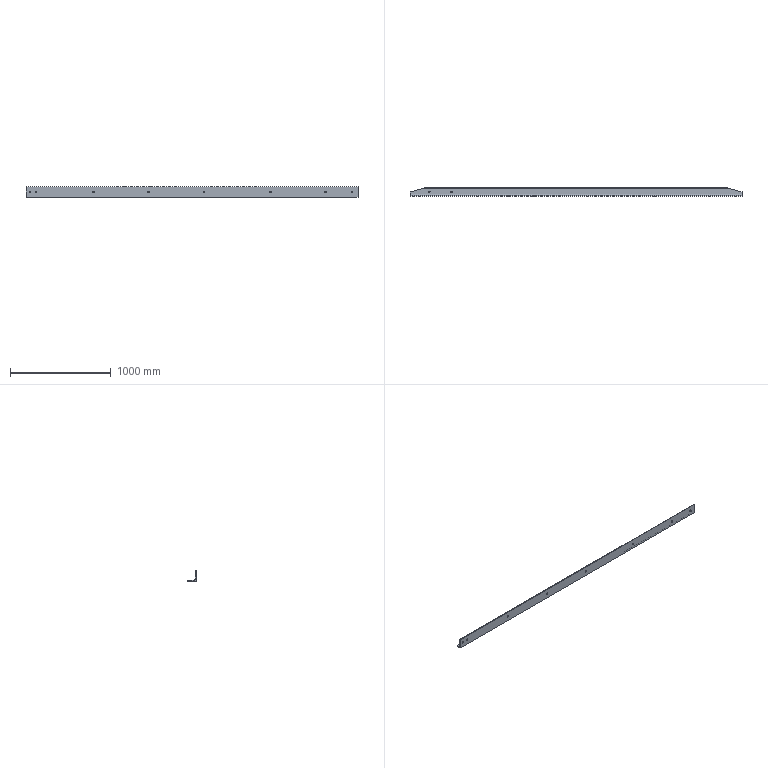Part | SolidWorks | features Chamfer 2, ICE 2, WeldMemberFeat 1, WeldmentFeature 1 | 1 solid | 33 faces | box 3300 x 80 x 100 mm | volume 4536810 mm3 | cylinder 23 | plane 10 | commonest cylinder face diameters 18 x20 5.333 x2 20 x1
STEP:
#1=CARTESIAN_POINT('',(-1469.,40.,8.));
#2=VERTEX_POINT('',#1);
#3=CARTESIAN_POINT('',(-1451.,40.,8.));
#4=VERTEX_POINT('',#3);
#5=CARTESIAN_POINT('',(-1460.,40.,8.));
#6=DIRECTION('',(0.,0.,1.));
#7=DIRECTION('',(0.,1.,0.));
#8=AXIS2_PLACEMENT_3D('',#5,#6,#7);
#9=CIRCLE('',#8,9.);
#10=EDGE_CURVE('',#2,#4,#9,.T.);
#11=ORIENTED_EDGE('',*,*,#10,.T.);
#12=CARTESIAN_POINT('',(-1451.,40.,0.));
#13=VERTEX_POINT('',#12);
#14=CARTESIAN_POINT('',(-1451.,40.,100.001));
#15=DIRECTION('',(0.,0.,-1.));
#16=VECTOR('',#15,1000.);
#17=LINE('',#14,#16);
#18=EDGE_CURVE('',#4,#13,#17,.T.);
#19=ORIENTED_EDGE('',*,*,#18,.T.);
#20=CARTESIAN_POINT('',(-1469.,40.,0.));
#21=VERTEX_POINT('',#20);
#22=CARTESIAN_POINT('',(-1460.,40.,0.));
#23=DIRECTION('',(0.,0.,-1.));
#24=DIRECTION('',(-1.,0.,0.));
#25=AXIS2_PLACEMENT_3D('',#22,#23,#24);
#26=CIRCLE('',#25,9.);
#27=EDGE_CURVE('',#13,#21,#26,.T.);
#28=ORIENTED_EDGE('',*,*,#27,.T.);
#29=CARTESIAN_POINT('',(-1469.,40.,100.001));
#30=DIRECTION('',(0.,0.,-1.));
#31=VECTOR('',#30,1000.);
#32=LINE('',#29,#31);
#33=EDGE_CURVE('',#2,#21,#32,.T.);
#34=ORIENTED_EDGE('',*,*,#33,.F.);
#35=EDGE_LOOP('',(#11,#19,#28,#34));
#36=FACE_OUTER_BOUND('',#35,.T.);
#37=CARTESIAN_POINT('',(-1460.,40.,100.001));
#38=DIRECTION('',(0.,0.,-1.));
#39=DIRECTION('',(-1.,0.,0.));
#40=AXIS2_PLACEMENT_3D('',#37,#38,#39);
#41=CYLINDRICAL_SURFACE('',#40,9.);
#42=ADVANCED_FACE('',(#36),#41,.F.);
#43=CARTESIAN_POINT('',(-1249.,40.,8.));
#44=VERTEX_POINT('',#43);
#45=CARTESIAN_POINT('',(-1231.,40.,8.));
#46=VERTEX_POINT('',#45);
#47=CARTESIAN_POINT('',(-1240.,40.,8.));
#48=DIRECTION('',(0.,0.,1.));
#49=DIRECTION('',(0.,1.,0.));
#50=AXIS2_PLACEMENT_3D('',#47,#48,#49);
#51=CIRCLE('',#50,9.);
#52=EDGE_CURVE('',#44,#46,#51,.T.);
#53=ORIENTED_EDGE('',*,*,#52,.T.);
#54=CARTESIAN_POINT('',(-1231.,40.,0.));
#55=VERTEX_POINT('',#54);
#56=CARTESIAN_POINT('',(-1231.,40.,100.001));
#57=DIRECTION('',(0.,0.,-1.));
#58=VECTOR('',#57,1000.);
#59=LINE('',#56,#58);
#60=EDGE_CURVE('',#46,#55,#59,.T.);
#61=ORIENTED_EDGE('',*,*,#60,.T.);
#62=CARTESIAN_POINT('',(-1249.,40.,0.));
#63=VERTEX_POINT('',#62);
#64=CARTESIAN_POINT('',(-1240.,40.,0.));
#65=DIRECTION('',(0.,0.,-1.));
#66=DIRECTION('',(-1.,0.,0.));
#67=AXIS2_PLACEMENT_3D('',#64,#65,#66);
#68=CIRCLE('',#67,9.);
#69=EDGE_CURVE('',#55,#63,#68,.T.);
#70=ORIENTED_EDGE('',*,*,#69,.T.);
#71=CARTESIAN_POINT('',(-1249.,40.,100.001));
#72=DIRECTION('',(0.,0.,-1.));
#73=VECTOR('',#72,1000.);
#74=LINE('',#71,#73);
#75=EDGE_CURVE('',#44,#63,#74,.T.);
#76=ORIENTED_EDGE('',*,*,#75,.F.);
#77=EDGE_LOOP('',(#53,#61,#70,#76));
#78=FACE_OUTER_BOUND('',#77,.T.);
#79=CARTESIAN_POINT('',(-1240.,40.,100.001));
#80=DIRECTION('',(0.,0.,-1.));
#81=DIRECTION('',(-1.,0.,0.));
#82=AXIS2_PLACEMENT_3D('',#79,#80,#81);
#83=CYLINDRICAL_SURFACE('',#82,9.);
#84=ADVANCED_FACE('',(#78),#83,.F.);
#85=CARTESIAN_POINT('',(-1601.,8.,50.));
#86=VERTEX_POINT('',#85);
#87=CARTESIAN_POINT('',(-1619.,8.,50.));
#88=VERTEX_POINT('',#87);
#89=CARTESIAN_POINT('',(-1610.,8.,50.));
#90=DIRECTION('',(0.,1.,0.));
#91=DIRECTION('',(0.,0.,-1.));
#92=AXIS2_PLACEMENT_3D('',#89,#90,#91);
#93=CIRCLE('',#92,9.);
#94=EDGE_CURVE('',#86,#88,#93,.T.);
#95=ORIENTED_EDGE('',*,*,#94,.T.);
#96=CARTESIAN_POINT('',(-1619.,0.,50.));
#97=VERTEX_POINT('',#96);
#98=CARTESIAN_POINT('',(-1619.,80.001,50.));
#99=DIRECTION('',(0.,-1.,0.));
#100=VECTOR('',#99,1000.);
#101=LINE('',#98,#100);
#102=EDGE_CURVE('',#88,#97,#101,.T.);
#103=ORIENTED_EDGE('',*,*,#102,.T.);
#104=CARTESIAN_POINT('',(-1601.,0.,50.));
#105=VERTEX_POINT('',#104);
#106=CARTESIAN_POINT('',(-1610.,0.,50.));
#107=DIRECTION('',(0.,-1.,0.));
#108=DIRECTION('',(1.,0.,0.));
#109=AXIS2_PLACEMENT_3D('',#106,#107,#108);
#110=CIRCLE('',#109,9.);
#111=EDGE_CURVE('',#97,#105,#110,.T.);
#112=ORIENTED_EDGE('',*,*,#111,.T.);
#113=CARTESIAN_POINT('',(-1601.,80.001,50.));
#114=DIRECTION('',(0.,-1.,0.));
#115=VECTOR('',#114,1000.);
#116=LINE('',#113,#115);
#117=EDGE_CURVE('',#86,#105,#116,.T.);
#118=ORIENTED_EDGE('',*,*,#117,.F.);
#119=EDGE_LOOP('',(#95,#103,#112,#118));
#120=FACE_OUTER_BOUND('',#119,.T.);
#121=CARTESIAN_POINT('',(-1610.,80.001,50.));
#122=DIRECTION('',(0.,-1.,0.));
#123=DIRECTION('',(1.,0.,0.));
#124=AXIS2_PLACEMENT_3D('',#121,#122,#123);
#125=CYLINDRICAL_SURFACE('',#124,9.);
#126=ADVANCED_FACE('',(#120),#125,.F.);
#127=CARTESIAN_POINT('',(-971.,8.,50.));
#128=VERTEX_POINT('',#127);
#129=CARTESIAN_POINT('',(-989.,8.,50.));
#130=VERTEX_POINT('',#129);
#131=CARTESIAN_POINT('',(-980.,8.,50.));
#132=DIRECTION('',(0.,1.,0.));
#133=DIRECTION('',(0.,0.,-1.));
#134=AXIS2_PLACEMENT_3D('',#131,#132,#133);
#135=CIRCLE('',#134,9.);
#136=EDGE_CURVE('',#128,#130,#135,.T.);
#137=ORIENTED_EDGE('',*,*,#136,.T.);
#138=CARTESIAN_POINT('',(-989.,0.,50.));
#139=VERTEX_POINT('',#138);
#140=CARTESIAN_POINT('',(-989.,80.001,50.));
#141=DIRECTION('',(0.,-1.,0.));
#142=VECTOR('',#141,1000.);
#143=LINE('',#140,#142);
#144=EDGE_CURVE('',#130,#139,#143,.T.);
#145=ORIENTED_EDGE('',*,*,#144,.T.);
#146=CARTESIAN_POINT('',(-971.,0.,50.));
#147=VERTEX_POINT('',#146);
#148=CARTESIAN_POINT('',(-980.,0.,50.));
#149=DIRECTION('',(0.,-1.,0.));
#150=DIRECTION('',(1.,0.,0.));
#151=AXIS2_PLACEMENT_3D('',#148,#149,#150);
#152=CIRCLE('',#151,9.);
#153=EDGE_CURVE('',#139,#147,#152,.T.);
#154=ORIENTED_EDGE('',*,*,#153,.T.);
#155=CARTESIAN_POINT('',(-971.,80.001,50.));
#156=DIRECTION('',(0.,-1.,0.));
#157=VECTOR('',#156,1000.);
#158=LINE('',#155,#157);
#159=EDGE_CURVE('',#128,#147,#158,.T.);
#160=ORIENTED_EDGE('',*,*,#159,.F.);
#161=EDGE_LOOP('',(#137,#145,#154,#160));
#162=FACE_OUTER_BOUND('',#161,.T.);
#163=CARTESIAN_POINT('',(-980.,80.001,50.));
#164=DIRECTION('',(0.,-1.,0.));
#165=DIRECTION('',(1.,0.,0.));
#166=AXIS2_PLACEMENT_3D('',#163,#164,#165);
#167=CYLINDRICAL_SURFACE('',#166,9.);
#168=ADVANCED_FACE('',(#162),#167,.F.);
#169=CARTESIAN_POINT('',(-421.,8.,50.));
#170=VERTEX_POINT('',#169);
#171=CARTESIAN_POINT('',(-439.,8.,50.));
#172=VERTEX_POINT('',#171);
#173=CARTESIAN_POINT('',(-430.,8.,50.));
#174=DIRECTION('',(0.,1.,0.));
#175=DIRECTION('',(0.,0.,-1.));
#176=AXIS2_PLACEMENT_3D('',#173,#174,#175);
#177=CIRCLE('',#176,9.);
#178=EDGE_CURVE('',#170,#172,#177,.T.);
#179=ORIENTED_EDGE('',*,*,#178,.T.);
#180=CARTESIAN_POINT('',(-439.,0.,50.));
#181=VERTEX_POINT('',#180);
#182=CARTESIAN_POINT('',(-439.,80.001,50.));
#183=DIRECTION('',(0.,-1.,0.));
#184=VECTOR('',#183,1000.);
#185=LINE('',#182,#184);
#186=EDGE_CURVE('',#172,#181,#185,.T.);
#187=ORIENTED_EDGE('',*,*,#186,.T.);
#188=CARTESIAN_POINT('',(-421.,0.,50.));
#189=VERTEX_POINT('',#188);
#190=CARTESIAN_POINT('',(-430.,0.,50.));
#191=DIRECTION('',(0.,-1.,0.));
#192=DIRECTION('',(1.,0.,0.));
#193=AXIS2_PLACEMENT_3D('',#190,#191,#192);
#194=CIRCLE('',#193,9.);
#195=EDGE_CURVE('',#181,#189,#194,.T.);
#196=ORIENTED_EDGE('',*,*,#195,.T.);
#197=CARTESIAN_POINT('',(-421.,80.001,50.));
#198=DIRECTION('',(0.,-1.,0.));
#199=VECTOR('',#198,1000.);
#200=LINE('',#197,#199);
#201=EDGE_CURVE('',#170,#189,#200,.T.);
#202=ORIENTED_EDGE('',*,*,#201,.F.);
#203=EDGE_LOOP('',(#179,#187,#196,#202));
#204=FACE_OUTER_BOUND('',#203,.T.);
#205=CARTESIAN_POINT('',(-430.,80.001,50.));
#206=DIRECTION('',(0.,-1.,0.));
#207=DIRECTION('',(1.,0.,0.));
#208=AXIS2_PLACEMENT_3D('',#205,#206,#207);
#209=CYLINDRICAL_SURFACE('',#208,9.);
#210=ADVANCED_FACE('',(#204),#209,.F.);
#211=CARTESIAN_POINT('',(129.,8.,50.));
#212=VERTEX_POINT('',#211);
#213=CARTESIAN_POINT('',(111.,8.,50.));
#214=VERTEX_POINT('',#213);
#215=CARTESIAN_POINT('',(120.,8.,50.));
#216=DIRECTION('',(0.,1.,0.));
#217=DIRECTION('',(0.,0.,-1.));
#218=AXIS2_PLACEMENT_3D('',#215,#216,#217);
#219=CIRCLE('',#218,9.);
#220=EDGE_CURVE('',#212,#214,#219,.T.);
#221=ORIENTED_EDGE('',*,*,#220,.T.);
#222=CARTESIAN_POINT('',(111.,0.,50.));
#223=VERTEX_POINT('',#222);
#224=CARTESIAN_POINT('',(111.,80.001,50.));
#225=DIRECTION('',(0.,-1.,0.));
#226=VECTOR('',#225,1000.);
#227=LINE('',#224,#226);
#228=EDGE_CURVE('',#214,#223,#227,.T.);
#229=ORIENTED_EDGE('',*,*,#228,.T.);
#230=CARTESIAN_POINT('',(129.,0.,50.));
#231=VERTEX_POINT('',#230);
#232=CARTESIAN_POINT('',(120.,0.,50.));
#233=DIRECTION('',(0.,-1.,0.));
#234=DIRECTION('',(1.,0.,0.));
#235=AXIS2_PLACEMENT_3D('',#232,#233,#234);
#236=CIRCLE('',#235,9.);
#237=EDGE_CURVE('',#223,#231,#236,.T.);
#238=ORIENTED_EDGE('',*,*,#237,.T.);
#239=CARTESIAN_POINT('',(129.,80.001,50.));
#240=DIRECTION('',(0.,-1.,0.));
#241=VECTOR('',#240,1000.);
#242=LINE('',#239,#241);
#243=EDGE_CURVE('',#212,#231,#242,.T.);
#244=ORIENTED_EDGE('',*,*,#243,.F.);
#245=EDGE_LOOP('',(#221,#229,#238,#244));
#246=FACE_OUTER_BOUND('',#245,.T.);
#247=CARTESIAN_POINT('',(120.,80.001,50.));
#248=DIRECTION('',(0.,-1.,0.));
#249=DIRECTION('',(1.,0.,0.));
#250=AXIS2_PLACEMENT_3D('',#247,#248,#249);
#251=CYLINDRICAL_SURFACE('',#250,9.);
#252=ADVANCED_FACE('',(#246),#251,.F.);
#253=CARTESIAN_POINT('',(-1541.,8.,50.));
#254=VERTEX_POINT('',#253);
#255=CARTESIAN_POINT('',(-1559.,8.,50.));
#256=VERTEX_POINT('',#255);
#257=CARTESIAN_POINT('',(-1550.,8.,50.));
#258=DIRECTION('',(0.,1.,0.));
#259=DIRECTION('',(0.,0.,-1.));
#260=AXIS2_PLACEMENT_3D('',#257,#258,#259);
#261=CIRCLE('',#260,9.);
#262=EDGE_CURVE('',#254,#256,#261,.T.);
#263=ORIENTED_EDGE('',*,*,#262,.T.);
#264=CARTESIAN_POINT('',(-1559.,0.,50.));
#265=VERTEX_POINT('',#264);
#266=CARTESIAN_POINT('',(-1559.,80.001,50.));
#267=DIRECTION('',(0.,-1.,0.));
#268=VECTOR('',#267,1000.);
#269=LINE('',#266,#268);
#270=EDGE_CURVE('',#256,#265,#269,.T.);
#271=ORIENTED_EDGE('',*,*,#270,.T.);
#272=CARTESIAN_POINT('',(-1541.,0.,50.));
#273=VERTEX_POINT('',#272);
#274=CARTESIAN_POINT('',(-1550.,0.,50.));
#275=DIRECTION('',(0.,-1.,0.));
#276=DIRECTION('',(1.,0.,0.));
#277=AXIS2_PLACEMENT_3D('',#274,#275,#276);
#278=CIRCLE('',#277,9.);
#279=EDGE_CURVE('',#265,#273,#278,.T.);
#280=ORIENTED_EDGE('',*,*,#279,.T.);
#281=CARTESIAN_POINT('',(-1541.,80.001,50.));
#282=DIRECTION('',(0.,-1.,0.));
#283=VECTOR('',#282,1000.);
#284=LINE('',#281,#283);
#285=EDGE_CURVE('',#254,#273,#284,.T.);
#286=ORIENTED_EDGE('',*,*,#285,.F.);
#287=EDGE_LOOP('',(#263,#271,#280,#286));
#288=FACE_OUTER_BOUND('',#287,.T.);
#289=CARTESIAN_POINT('',(-1550.,80.001,50.));
#290=DIRECTION('',(0.,-1.,0.));
#291=DIRECTION('',(1.,0.,0.));
#292=AXIS2_PLACEMENT_3D('',#289,#290,#291);
#293=CYLINDRICAL_SURFACE('',#292,9.);
#294=ADVANCED_FACE('',(#288),#293,.F.);
#295=CARTESIAN_POINT('',(1599.,8.,50.));
#296=VERTEX_POINT('',#295);
#297=CARTESIAN_POINT('',(1581.,8.,50.));
#298=VERTEX_POINT('',#297);
#299=CARTESIAN_POINT('',(1590.,8.,50.));
#300=DIRECTION('',(0.,1.,0.));
#301=DIRECTION('',(0.,0.,-1.));
#302=AXIS2_PLACEMENT_3D('',#299,#300,#301);
#303=CIRCLE('',#302,9.);
#304=EDGE_CURVE('',#296,#298,#303,.T.);
#305=ORIENTED_EDGE('',*,*,#304,.T.);
#306=CARTESIAN_POINT('',(1581.,0.,50.));
#307=VERTEX_POINT('',#306);
#308=CARTESIAN_POINT('',(1581.,80.001,50.));
#309=DIRECTION('',(0.,-1.,0.));
#310=VECTOR('',#309,1000.);
#311=LINE('',#308,#310);
#312=EDGE_CURVE('',#298,#307,#311,.T.);
#313=ORIENTED_EDGE('',*,*,#312,.T.);
#314=CARTESIAN_POINT('',(1599.,0.,50.));
#315=VERTEX_POINT('',#314);
#316=CARTESIAN_POINT('',(1590.,0.,50.));
#317=DIRECTION('',(0.,-1.,0.));
#318=DIRECTION('',(1.,0.,0.));
#319=AXIS2_PLACEMENT_3D('',#316,#317,#318);
#320=CIRCLE('',#319,9.);
#321=EDGE_CURVE('',#307,#315,#320,.T.);
#322=ORIENTED_EDGE('',*,*,#321,.T.);
#323=CARTESIAN_POINT('',(1599.,80.001,50.));
#324=DIRECTION('',(0.,-1.,0.));
#325=VECTOR('',#324,1000.);
#326=LINE('',#323,#325);
#327=EDGE_CURVE('',#296,#315,#326,.T.);
#328=ORIENTED_EDGE('',*,*,#327,.F.);
#329=EDGE_LOOP('',(#305,#313,#322,#328));
#330=FACE_OUTER_BOUND('',#329,.T.);
#331=CARTESIAN_POINT('',(1590.,80.001,50.));
#332=DIRECTION('',(0.,-1.,0.));
#333=DIRECTION('',(1.,0.,0.));
#334=AXIS2_PLACEMENT_3D('',#331,#332,#333);
#335=CYLINDRICAL_SURFACE('',#334,9.);
#336=ADVANCED_FACE('',(#330),#335,.F.);
#337=CARTESIAN_POINT('',(1339.,8.,50.));
#338=VERTEX_POINT('',#337);
#339=CARTESIAN_POINT('',(1321.,8.,50.));
#340=VERTEX_POINT('',#339);
#341=CARTESIAN_POINT('',(1330.,8.,50.));
#342=DIRECTION('',(0.,1.,0.));
#343=DIRECTION('',(0.,0.,-1.));
#344=AXIS2_PLACEMENT_3D('',#341,#342,#343);
#345=CIRCLE('',#344,9.);
#346=EDGE_CURVE('',#338,#340,#345,.T.);
#347=ORIENTED_EDGE('',*,*,#346,.T.);
#348=CARTESIAN_POINT('',(1321.,0.,50.));
#349=VERTEX_POINT('',#348);
#350=CARTESIAN_POINT('',(1321.,80.001,50.));
#351=DIRECTION('',(0.,-1.,0.));
#352=VECTOR('',#351,1000.);
#353=LINE('',#350,#352);
#354=EDGE_CURVE('',#340,#349,#353,.T.);
#355=ORIENTED_EDGE('',*,*,#354,.T.);
#356=CARTESIAN_POINT('',(1339.,0.,50.));
#357=VERTEX_POINT('',#356);
#358=CARTESIAN_POINT('',(1330.,0.,50.));
#359=DIRECTION('',(0.,-1.,0.));
#360=DIRECTION('',(1.,0.,0.));
#361=AXIS2_PLACEMENT_3D('',#358,#359,#360);
#362=CIRCLE('',#361,9.);
#363=EDGE_CURVE('',#349,#357,#362,.T.);
#364=ORIENTED_EDGE('',*,*,#363,.T.);
#365=CARTESIAN_POINT('',(1339.,80.001,50.));
#366=DIRECTION('',(0.,-1.,0.));
#367=VECTOR('',#366,1000.);
#368=LINE('',#365,#367);
#369=EDGE_CURVE('',#338,#357,#368,.T.);
#370=ORIENTED_EDGE('',*,*,#369,.F.);
#371=EDGE_LOOP('',(#347,#355,#364,#370));
#372=FACE_OUTER_BOUND('',#371,.T.);
#373=CARTESIAN_POINT('',(1330.,80.001,50.));
#374=DIRECTION('',(0.,-1.,0.));
#375=DIRECTION('',(1.,0.,0.));
#376=AXIS2_PLACEMENT_3D('',#373,#374,#375);
#377=CYLINDRICAL_SURFACE('',#376,9.);
#378=ADVANCED_FACE('',(#372),#377,.F.);
#379=CARTESIAN_POINT('',(789.,8.,50.));
#380=VERTEX_POINT('',#379);
#381=CARTESIAN_POINT('',(771.,8.,50.));
#382=VERTEX_POINT('',#381);
#383=CARTESIAN_POINT('',(780.,8.,50.));
#384=DIRECTION('',(0.,1.,0.));
#385=DIRECTION('',(0.,0.,-1.));
#386=AXIS2_PLACEMENT_3D('',#383,#384,#385);
#387=CIRCLE('',#386,9.);
#388=EDGE_CURVE('',#380,#382,#387,.T.);
#389=ORIENTED_EDGE('',*,*,#388,.T.);
#390=CARTESIAN_POINT('',(771.,0.,50.));
#391=VERTEX_POINT('',#390);
#392=CARTESIAN_POINT('',(771.,80.001,50.));
#393=DIRECTION('',(0.,-1.,0.));
#394=VECTOR('',#393,1000.);
#395=LINE('',#392,#394);
#396=EDGE_CURVE('',#382,#391,#395,.T.);
#397=ORIENTED_EDGE('',*,*,#396,.T.);
#398=CARTESIAN_POINT('',(789.,0.,50.));
#399=VERTEX_POINT('',#398);
#400=CARTESIAN_POINT('',(780.,0.,50.));
#401=DIRECTION('',(0.,-1.,0.));
#402=DIRECTION('',(1.,0.,0.));
#403=AXIS2_PLACEMENT_3D('',#400,#401,#402);
#404=CIRCLE('',#403,9.);
#405=EDGE_CURVE('',#391,#399,#404,.T.);
#406=ORIENTED_EDGE('',*,*,#405,.T.);
#407=CARTESIAN_POINT('',(789.,80.001,50.));
#408=DIRECTION('',(0.,-1.,0.));
#409=VECTOR('',#408,1000.);
#410=LINE('',#407,#409);
#411=EDGE_CURVE('',#380,#399,#410,.T.);
#412=ORIENTED_EDGE('',*,*,#411,.F.);
#413=EDGE_LOOP('',(#389,#397,#406,#412));
#414=FACE_OUTER_BOUND('',#413,.T.);
#415=CARTESIAN_POINT('',(780.,80.001,50.));
#416=DIRECTION('',(0.,-1.,0.));
#417=DIRECTION('',(1.,0.,0.));
#418=AXIS2_PLACEMENT_3D('',#415,#416,#417);
#419=CYLINDRICAL_SURFACE('',#418,9.);
#420=ADVANCED_FACE('',(#414),#419,.F.);
#421=CARTESIAN_POINT('',(-1650.,18.,8.));
#422=VERTEX_POINT('',#421);
#423=CARTESIAN_POINT('',(-1650.,8.,18.));
#424=VERTEX_POINT('',#423);
#425=CARTESIAN_POINT('',(-1650.,18.,18.));
#426=DIRECTION('',(-1.,0.,0.));
#427=DIRECTION('',(0.,0.,-1.));
#428=AXIS2_PLACEMENT_3D('',#425,#426,#427);
#429=CIRCLE('',#428,10.);
#430=EDGE_CURVE('',#422,#424,#429,.T.);
#431=ORIENTED_EDGE('',*,*,#430,.T.);
#432=CARTESIAN_POINT('',(1650.,8.,18.));
#433=VERTEX_POINT('',#432);
#434=CARTESIAN_POINT('',(1650.,8.,18.));
#435=DIRECTION('',(-1.,0.,0.));
#436=VECTOR('',#435,1000.);
#437=LINE('',#434,#436);
#438=EDGE_CURVE('',#433,#424,#437,.T.);
#439=ORIENTED_EDGE('',*,*,#438,.F.);
#440=CARTESIAN_POINT('',(1650.,18.,8.));
#441=VERTEX_POINT('',#440);
#442=CARTESIAN_POINT('',(1650.,18.,18.));
#443=DIRECTION('',(-1.,0.,0.));
#444=DIRECTION('',(0.,0.,-1.));
#445=AXIS2_PLACEMENT_3D('',#442,#443,#444);
#446=CIRCLE('',#445,10.);
#447=EDGE_CURVE('',#441,#433,#446,.T.);
#448=ORIENTED_EDGE('',*,*,#447,.F.);
#449=CARTESIAN_POINT('',(1650.,18.,8.));
#450=DIRECTION('',(-1.,0.,0.));
#451=VECTOR('',#450,1000.);
#452=LINE('',#449,#451);
#453=EDGE_CURVE('',#441,#422,#452,.T.);
#454=ORIENTED_EDGE('',*,*,#453,.T.);
#455=EDGE_LOOP('',(#431,#439,#448,#454));
#456=FACE_OUTER_BOUND('',#455,.T.);
#457=CARTESIAN_POINT('',(1650.,18.,18.));
#458=DIRECTION('',(-1.,0.,0.));
#459=DIRECTION('',(0.,0.,1.));
#460=AXIS2_PLACEMENT_3D('',#457,#458,#459);
#461=CYLINDRICAL_SURFACE('',#460,10.);
#462=ADVANCED_FACE('',(#456),#461,.F.);
#463=ORIENTED_EDGE('',*,*,#94,.F.);
#464=CARTESIAN_POINT('',(-1610.,8.,50.));
#465=DIRECTION('',(0.,1.,0.));
#466=DIRECTION('',(0.,0.,-1.));
#467=AXIS2_PLACEMENT_3D('',#464,#465,#466);
#468=CIRCLE('',#467,9.);
#469=EDGE_CURVE('',#88,#86,#468,.T.);
#470=ORIENTED_EDGE('',*,*,#469,.F.);
#471=EDGE_LOOP('',(#463,#470));
#472=FACE_BOUND('',#471,.T.);
#473=ORIENTED_EDGE('',*,*,#136,.F.);
#474=CARTESIAN_POINT('',(-980.,8.,50.));
#475=DIRECTION('',(0.,1.,0.));
#476=DIRECTION('',(0.,0.,-1.));
#477=AXIS2_PLACEMENT_3D('',#474,#475,#476);
#478=CIRCLE('',#477,9.);
#479=EDGE_CURVE('',#130,#128,#478,.T.);
#480=ORIENTED_EDGE('',*,*,#479,.F.);
#481=EDGE_LOOP('',(#473,#480));
#482=FACE_BOUND('',#481,.T.);
#483=ORIENTED_EDGE('',*,*,#178,.F.);
#484=CARTESIAN_POINT('',(-430.,8.,50.));
#485=DIRECTION('',(0.,1.,0.));
#486=DIRECTION('',(0.,0.,-1.));
#487=AXIS2_PLACEMENT_3D('',#484,#485,#486);
#488=CIRCLE('',#487,9.);
#489=EDGE_CURVE('',#172,#170,#488,.T.);
#490=ORIENTED_EDGE('',*,*,#489,.F.);
#491=EDGE_LOOP('',(#483,#490));
#492=FACE_BOUND('',#491,.T.);
#493=ORIENTED_EDGE('',*,*,#220,.F.);
#494=CARTESIAN_POINT('',(120.,8.,50.));
#495=DIRECTION('',(0.,1.,0.));
#496=DIRECTION('',(0.,0.,-1.));
#497=AXIS2_PLACEMENT_3D('',#494,#495,#496);
#498=CIRCLE('',#497,9.);
#499=EDGE_CURVE('',#214,#212,#498,.T.);
#500=ORIENTED_EDGE('',*,*,#499,.F.);
#501=EDGE_LOOP('',(#493,#500));
#502=FACE_BOUND('',#501,.T.);
#503=ORIENTED_EDGE('',*,*,#262,.F.);
#504=CARTESIAN_POINT('',(-1550.,8.,50.));
#505=DIRECTION('',(0.,1.,0.));
#506=DIRECTION('',(0.,0.,-1.));
#507=AXIS2_PLACEMENT_3D('',#504,#505,#506);
#508=CIRCLE('',#507,9.);
#509=EDGE_CURVE('',#256,#254,#508,.T.);
#510=ORIENTED_EDGE('',*,*,#509,.F.);
#511=EDGE_LOOP('',(#503,#510));
#512=FACE_BOUND('',#511,.T.);
#513=ORIENTED_EDGE('',*,*,#304,.F.);
#514=CARTESIAN_POINT('',(1590.,8.,50.));
#515=DIRECTION('',(0.,1.,0.));
#516=DIRECTION('',(0.,0.,-1.));
#517=AXIS2_PLACEMENT_3D('',#514,#515,#516);
#518=CIRCLE('',#517,9.);
#519=EDGE_CURVE('',#298,#296,#518,.T.);
#520=ORIENTED_EDGE('',*,*,#519,.F.);
#521=EDGE_LOOP('',(#513,#520));
#522=FACE_BOUND('',#521,.T.);
#523=ORIENTED_EDGE('',*,*,#346,.F.);
#524=CARTESIAN_POINT('',(1330.,8.,50.));
#525=DIRECTION('',(0.,1.,0.));
#526=DIRECTION('',(0.,0.,-1.));
#527=AXIS2_PLACEMENT_3D('',#524,#525,#526);
#528=CIRCLE('',#527,9.);
#529=EDGE_CURVE('',#340,#338,#528,.T.);
#530=ORIENTED_EDGE('',*,*,#529,.F.);
#531=EDGE_LOOP('',(#523,#530));
#532=FACE_BOUND('',#531,.T.);
#533=ORIENTED_EDGE('',*,*,#388,.F.);
#534=CARTESIAN_POINT('',(780.,8.,50.));
#535=DIRECTION('',(0.,1.,0.));
#536=DIRECTION('',(0.,0.,-1.));
#537=AXIS2_PLACEMENT_3D('',#534,#535,#536);
#538=CIRCLE('',#537,9.);
#539=EDGE_CURVE('',#382,#380,#538,.T.);
#540=ORIENTED_EDGE('',*,*,#539,.F.);
#541=EDGE_LOOP('',(#533,#540));
#542=FACE_BOUND('',#541,.T.);
#543=CARTESIAN_POINT('',(-1650.,8.,97.333));
#544=VERTEX_POINT('',#543);
#545=CARTESIAN_POINT('',(-1650.,8.,97.333));
#546=DIRECTION('',(0.,0.,1.));
#547=VECTOR('',#546,1000.);
#548=LINE('',#545,#547);
#549=EDGE_CURVE('',#424,#544,#548,.T.);
#550=ORIENTED_EDGE('',*,*,#549,.T.);
#551=CARTESIAN_POINT('',(1650.,8.,97.333));
#552=VERTEX_POINT('',#551);
#553=CARTESIAN_POINT('',(1650.,8.,97.333));
#554=DIRECTION('',(-1.,0.,0.));
#555=VECTOR('',#554,1000.);
#556=LINE('',#553,#555);
#557=EDGE_CURVE('',#552,#544,#556,.T.);
#558=ORIENTED_EDGE('',*,*,#557,.F.);
#559=CARTESIAN_POINT('',(1650.,8.,97.333));
#560=DIRECTION('',(0.,0.,1.));
#561=VECTOR('',#560,1000.);
#562=LINE('',#559,#561);
#563=EDGE_CURVE('',#433,#552,#562,.T.);
#564=ORIENTED_EDGE('',*,*,#563,.F.);
#565=ORIENTED_EDGE('',*,*,#438,.T.);
#566=EDGE_LOOP('',(#550,#558,#564,#565));
#567=FACE_OUTER_BOUND('',#566,.T.);
#568=CARTESIAN_POINT('',(1650.,8.,97.333));
#569=DIRECTION('',(0.,-1.,0.));
#570=DIRECTION('',(0.,0.,-1.));
#571=AXIS2_PLACEMENT_3D('',#568,#569,#570);
#572=PLANE('',#571);
#573=ADVANCED_FACE('',(#472,#482,#492,#502,#512,#522,#532,#542,#567),#572,.F.);
#574=CARTESIAN_POINT('',(-1650.,5.333,100.));
#575=VERTEX_POINT('',#574);
#576=CARTESIAN_POINT('',(-1650.,5.333,97.333));
#577=DIRECTION('',(1.,0.,0.));
#578=DIRECTION('',(0.,0.,1.));
#579=AXIS2_PLACEMENT_3D('',#576,#577,#578);
#580=CIRCLE('',#579,2.667);
#581=EDGE_CURVE('',#544,#575,#580,.T.);
#582=ORIENTED_EDGE('',*,*,#581,.T.);
#583=CARTESIAN_POINT('',(1650.,5.333,100.));
#584=VERTEX_POINT('',#583);
#585=CARTESIAN_POINT('',(1650.,5.333,100.));
#586=DIRECTION('',(-1.,0.,0.));
#587=VECTOR('',#586,1000.);
#588=LINE('',#585,#587);
#589=EDGE_CURVE('',#584,#575,#588,.T.);
#590=ORIENTED_EDGE('',*,*,#589,.F.);
#591=CARTESIAN_POINT('',(1650.,5.333,97.333));
#592=DIRECTION('',(1.,0.,0.));
#593=DIRECTION('',(0.,0.,1.));
#594=AXIS2_PLACEMENT_3D('',#591,#592,#593);
#595=CIRCLE('',#594,2.667);
#596=EDGE_CURVE('',#552,#584,#595,.T.);
#597=ORIENTED_EDGE('',*,*,#596,.F.);
#598=ORIENTED_EDGE('',*,*,#557,.T.);
#599=EDGE_LOOP('',(#582,#590,#597,#598));
#600=FACE_OUTER_BOUND('',#599,.T.);
#601=CARTESIAN_POINT('',(1650.,5.333,97.333));
#602=DIRECTION('',(-1.,0.,0.));
#603=DIRECTION('',(0.,0.,1.));
#604=AXIS2_PLACEMENT_3D('',#601,#602,#603);
#605=CYLINDRICAL_SURFACE('',#604,2.667);
#606=ADVANCED_FACE('',(#600),#605,.T.);
#607=CARTESIAN_POINT('',(-1650.,0.,100.));
#608=VERTEX_POINT('',#607);
#609=CARTESIAN_POINT('',(-1650.,0.,100.));
#610=DIRECTION('',(0.,-1.,0.));
#611=VECTOR('',#610,1000.);
#612=LINE('',#609,#611);
#613=EDGE_CURVE('',#575,#608,#612,.T.);
#614=ORIENTED_EDGE('',*,*,#613,.T.);
#615=CARTESIAN_POINT('',(1650.,0.,100.));
#616=VERTEX_POINT('',#615);
#617=CARTESIAN_POINT('',(1650.,0.,100.));
#618=DIRECTION('',(-1.,0.,0.));
#619=VECTOR('',#618,1000.);
#620=LINE('',#617,#619);
#621=EDGE_CURVE('',#616,#608,#620,.T.);
#622=ORIENTED_EDGE('',*,*,#621,.F.);
#623=CARTESIAN_POINT('',(1650.,0.,100.));
#624=DIRECTION('',(0.,-1.,0.));
#625=VECTOR('',#624,1000.);
#626=LINE('',#623,#625);
#627=EDGE_CURVE('',#584,#616,#626,.T.);
#628=ORIENTED_EDGE('',*,*,#627,.F.);
#629=ORIENTED_EDGE('',*,*,#589,.T.);
#630=EDGE_LOOP('',(#614,#622,#628,#629));
#631=FACE_OUTER_BOUND('',#630,.T.);
#632=CARTESIAN_POINT('',(1650.,0.,100.));
#633=DIRECTION('',(0.,0.,-1.));
#634=DIRECTION('',(0.,1.,0.));
#635=AXIS2_PLACEMENT_3D('',#632,#633,#634);
#636=PLANE('',#635);
#637=ADVANCED_FACE('',(#631),#636,.F.);
#638=CARTESIAN_POINT('',(-1610.,0.,50.));
#639=DIRECTION('',(0.,-1.,0.));
#640=DIRECTION('',(1.,0.,0.));
#641=AXIS2_PLACEMENT_3D('',#638,#639,#640);
#642=CIRCLE('',#641,9.);
#643=EDGE_CURVE('',#105,#97,#642,.T.);
#644=ORIENTED_EDGE('',*,*,#643,.F.);
#645=ORIENTED_EDGE('',*,*,#111,.F.);
#646=EDGE_LOOP('',(#644,#645));
#647=FACE_BOUND('',#646,.T.);
#648=CARTESIAN_POINT('',(-980.,0.,50.));
#649=DIRECTION('',(0.,-1.,0.));
#650=DIRECTION('',(1.,0.,0.));
#651=AXIS2_PLACEMENT_3D('',#648,#649,#650);
#652=CIRCLE('',#651,9.);
#653=EDGE_CURVE('',#147,#139,#652,.T.);
#654=ORIENTED_EDGE('',*,*,#653,.F.);
#655=ORIENTED_EDGE('',*,*,#153,.F.);
#656=EDGE_LOOP('',(#654,#655));
#657=FACE_BOUND('',#656,.T.);
#658=CARTESIAN_POINT('',(-430.,0.,50.));
#659=DIRECTION('',(0.,-1.,0.));
#660=DIRECTION('',(1.,0.,0.));
#661=AXIS2_PLACEMENT_3D('',#658,#659,#660);
#662=CIRCLE('',#661,9.);
#663=EDGE_CURVE('',#189,#181,#662,.T.);
#664=ORIENTED_EDGE('',*,*,#663,.F.);
#665=ORIENTED_EDGE('',*,*,#195,.F.);
#666=EDGE_LOOP('',(#664,#665));
#667=FACE_BOUND('',#666,.T.);
#668=CARTESIAN_POINT('',(120.,0.,50.));
#669=DIRECTION('',(0.,-1.,0.));
#670=DIRECTION('',(1.,0.,0.));
#671=AXIS2_PLACEMENT_3D('',#668,#669,#670);
#672=CIRCLE('',#671,9.);
#673=EDGE_CURVE('',#231,#223,#672,.T.);
#674=ORIENTED_EDGE('',*,*,#673,.F.);
#675=ORIENTED_EDGE('',*,*,#237,.F.);
#676=EDGE_LOOP('',(#674,#675));
#677=FACE_BOUND('',#676,.T.);
#678=CARTESIAN_POINT('',(-1550.,0.,50.));
#679=DIRECTION('',(0.,-1.,0.));
#680=DIRECTION('',(1.,0.,0.));
#681=AXIS2_PLACEMENT_3D('',#678,#679,#680);
#682=CIRCLE('',#681,9.);
#683=EDGE_CURVE('',#273,#265,#682,.T.);
#684=ORIENTED_EDGE('',*,*,#683,.F.);
#685=ORIENTED_EDGE('',*,*,#279,.F.);
#686=EDGE_LOOP('',(#684,#685));
#687=FACE_BOUND('',#686,.T.);
#688=CARTESIAN_POINT('',(1590.,0.,50.));
#689=DIRECTION('',(0.,-1.,0.));
#690=DIRECTION('',(1.,0.,0.));
#691=AXIS2_PLACEMENT_3D('',#688,#689,#690);
#692=CIRCLE('',#691,9.);
#693=EDGE_CURVE('',#315,#307,#692,.T.);
#694=ORIENTED_EDGE('',*,*,#693,.F.);
#695=ORIENTED_EDGE('',*,*,#321,.F.);
#696=EDGE_LOOP('',(#694,#695));
#697=FACE_BOUND('',#696,.T.);
#698=CARTESIAN_POINT('',(1330.,0.,50.));
#699=DIRECTION('',(0.,-1.,0.));
#700=DIRECTION('',(1.,0.,0.));
#701=AXIS2_PLACEMENT_3D('',#698,#699,#700);
#702=CIRCLE('',#701,9.);
#703=EDGE_CURVE('',#357,#349,#702,.T.);
#704=ORIENTED_EDGE('',*,*,#703,.F.);
#705=ORIENTED_EDGE('',*,*,#363,.F.);
#706=EDGE_LOOP('',(#704,#705));
#707=FACE_BOUND('',#706,.T.);
#708=CARTESIAN_POINT('',(780.,0.,50.));
#709=DIRECTION('',(0.,-1.,0.));
#710=DIRECTION('',(1.,0.,0.));
#711=AXIS2_PLACEMENT_3D('',#708,#709,#710);
#712=CIRCLE('',#711,9.);
#713=EDGE_CURVE('',#399,#391,#712,.T.);
#714=ORIENTED_EDGE('',*,*,#713,.F.);
#715=ORIENTED_EDGE('',*,*,#405,.F.);
#716=EDGE_LOOP('',(#714,#715));
#717=FACE_BOUND('',#716,.T.);
#718=CARTESIAN_POINT('',(-1650.,0.,0.));
#719=VERTEX_POINT('',#718);
#720=CARTESIAN_POINT('',(-1650.,0.,100.));
#721=DIRECTION('',(0.,0.,-1.));
#722=VECTOR('',#721,1000.);
#723=LINE('',#720,#722);
#724=EDGE_CURVE('',#608,#719,#723,.T.);
#725=ORIENTED_EDGE('',*,*,#724,.T.);
#726=CARTESIAN_POINT('',(1650.,0.,0.));
#727=VERTEX_POINT('',#726);
#728=CARTESIAN_POINT('',(1650.,0.,0.));
#729=DIRECTION('',(-1.,0.,0.));
#730=VECTOR('',#729,1000.);
#731=LINE('',#728,#730);
#732=EDGE_CURVE('',#727,#719,#731,.T.);
#733=ORIENTED_EDGE('',*,*,#732,.F.);
#734=CARTESIAN_POINT('',(1650.,0.,100.));
#735=DIRECTION('',(0.,0.,-1.));
#736=VECTOR('',#735,1000.);
#737=LINE('',#734,#736);
#738=EDGE_CURVE('',#616,#727,#737,.T.);
#739=ORIENTED_EDGE('',*,*,#738,.F.);
#740=ORIENTED_EDGE('',*,*,#621,.T.);
#741=EDGE_LOOP('',(#725,#733,#739,#740));
#742=FACE_OUTER_BOUND('',#741,.T.);
#743=CARTESIAN_POINT('',(1650.,0.,100.));
#744=DIRECTION('',(0.,1.,0.));
#745=DIRECTION('',(0.,0.,1.));
#746=AXIS2_PLACEMENT_3D('',#743,#744,#745);
#747=PLANE('',#746);
#748=ADVANCED_FACE('',(#647,#657,#667,#677,#687,#697,#707,#717,#742),#747,.F.);
#749=CARTESIAN_POINT('',(-1460.,40.,0.));
#750=DIRECTION('',(0.,0.,-1.));
#751=DIRECTION('',(-1.,0.,0.));
#752=AXIS2_PLACEMENT_3D('',#749,#750,#751);
#753=CIRCLE('',#752,9.);
#754=EDGE_CURVE('',#21,#13,#753,.T.);
#755=ORIENTED_EDGE('',*,*,#754,.F.);
#756=ORIENTED_EDGE('',*,*,#27,.F.);
#757=EDGE_LOOP('',(#755,#756));
#758=FACE_BOUND('',#757,.T.);
#759=CARTESIAN_POINT('',(-1240.,40.,0.));
#760=DIRECTION('',(0.,0.,-1.));
#761=DIRECTION('',(-1.,0.,0.));
#762=AXIS2_PLACEMENT_3D('',#759,#760,#761);
#763=CIRCLE('',#762,9.);
#764=EDGE_CURVE('',#63,#55,#763,.T.);
#765=ORIENTED_EDGE('',*,*,#764,.F.);
#766=ORIENTED_EDGE('',*,*,#69,.F.);
#767=EDGE_LOOP('',(#765,#766));
#768=FACE_BOUND('',#767,.T.);
#769=CARTESIAN_POINT('',(1510.,80.,0.));
#770=VERTEX_POINT('',#769);
#771=CARTESIAN_POINT('',(-1510.,80.,0.));
#772=VERTEX_POINT('',#771);
#773=CARTESIAN_POINT('',(1650.,80.,0.));
#774=DIRECTION('',(-1.,0.,0.));
#775=VECTOR('',#774,1000.);
#776=LINE('',#773,#775);
#777=EDGE_CURVE('',#770,#772,#776,.T.);
#778=ORIENTED_EDGE('',*,*,#777,.F.);
#779=CARTESIAN_POINT('',(1650.,40.,0.));
#780=VERTEX_POINT('',#779);
#781=CARTESIAN_POINT('',(1650.,40.,0.));
#782=DIRECTION('',(0.9615,-0.2747,0.));
#783=VECTOR('',#782,1000.);
#784=LINE('',#781,#783);
#785=EDGE_CURVE('',#770,#780,#784,.T.);
#786=ORIENTED_EDGE('',*,*,#785,.T.);
#787=CARTESIAN_POINT('',(1650.,0.,0.));
#788=DIRECTION('',(0.,1.,0.));
#789=VECTOR('',#788,1000.);
#790=LINE('',#787,#789);
#791=EDGE_CURVE('',#727,#780,#790,.T.);
#792=ORIENTED_EDGE('',*,*,#791,.F.);
#793=ORIENTED_EDGE('',*,*,#732,.T.);
#794=CARTESIAN_POINT('',(-1650.,40.,0.));
#795=VERTEX_POINT('',#794);
#796=CARTESIAN_POINT('',(-1650.,0.,0.));
#797=DIRECTION('',(0.,1.,0.));
#798=VECTOR('',#797,1000.);
#799=LINE('',#796,#798);
#800=EDGE_CURVE('',#719,#795,#799,.T.);
#801=ORIENTED_EDGE('',*,*,#800,.T.);
#802=CARTESIAN_POINT('',(-1510.,80.,0.));
#803=DIRECTION('',(0.9615,0.2747,0.));
#804=VECTOR('',#803,1000.);
#805=LINE('',#802,#804);
#806=EDGE_CURVE('',#795,#772,#805,.T.);
#807=ORIENTED_EDGE('',*,*,#806,.T.);
#808=EDGE_LOOP('',(#778,#786,#792,#793,#801,#807));
#809=FACE_OUTER_BOUND('',#808,.T.);
#810=CARTESIAN_POINT('',(1650.,0.,0.));
#811=DIRECTION('',(0.,0.,1.));
#812=DIRECTION('',(1.,0.,0.));
#813=AXIS2_PLACEMENT_3D('',#810,#811,#812);
#814=PLANE('',#813);
#815=ADVANCED_FACE('',(#758,#768,#809),#814,.F.);
#816=CARTESIAN_POINT('',(1510.,80.,5.333));
#817=VERTEX_POINT('',#816);
#818=CARTESIAN_POINT('',(-1510.,80.,5.333));
#819=VERTEX_POINT('',#818);
#820=CARTESIAN_POINT('',(1650.,80.,5.333));
#821=DIRECTION('',(-1.,0.,0.));
#822=VECTOR('',#821,1000.);
#823=LINE('',#820,#822);
#824=EDGE_CURVE('',#817,#819,#823,.T.);
#825=ORIENTED_EDGE('',*,*,#824,.F.);
#826=CARTESIAN_POINT('',(1510.,80.,0.));
#827=DIRECTION('',(0.,0.,-1.));
#828=VECTOR('',#827,1000.);
#829=LINE('',#826,#828);
#830=EDGE_CURVE('',#817,#770,#829,.T.);
#831=ORIENTED_EDGE('',*,*,#830,.T.);
#832=ORIENTED_EDGE('',*,*,#777,.T.);
#833=CARTESIAN_POINT('',(-1510.,80.,0.));
#834=DIRECTION('',(0.,0.,1.));
#835=VECTOR('',#834,1000.);
#836=LINE('',#833,#835);
#837=EDGE_CURVE('',#772,#819,#836,.T.);
#838=ORIENTED_EDGE('',*,*,#837,.T.);
#839=EDGE_LOOP('',(#825,#831,#832,#838));
#840=FACE_OUTER_BOUND('',#839,.T.);
#841=CARTESIAN_POINT('',(1650.,80.,0.));
#842=DIRECTION('',(0.,-1.,0.));
#843=DIRECTION('',(0.,0.,-1.));
#844=AXIS2_PLACEMENT_3D('',#841,#842,#843);
#845=PLANE('',#844);
#846=ADVANCED_FACE('',(#840),#845,.F.);
#847=CARTESIAN_POINT('',(1519.333,77.333,8.));
#848=VERTEX_POINT('',#847);
#849=CARTESIAN_POINT('',(-1519.333,77.333,8.));
#850=VERTEX_POINT('',#849);
#851=CARTESIAN_POINT('',(1650.,77.333,8.));
#852=DIRECTION('',(-1.,0.,0.));
#853=VECTOR('',#852,1000.);
#854=LINE('',#851,#853);
#855=EDGE_CURVE('',#848,#850,#854,.T.);
#856=ORIENTED_EDGE('',*,*,#855,.F.);
#857=CARTESIAN_POINT('',(1519.333,77.333,8.));
#858=CARTESIAN_POINT('',(1513.866,78.895,8.));
#859=CARTESIAN_POINT('',(1510.,80.,6.895));
#860=CARTESIAN_POINT('',(1510.,80.,5.333));
#861=(BOUNDED_CURVE()B_SPLINE_CURVE(3,(#857,#858,#859,#860),.UNSPECIFIED.,.F.,.F.)B_SPLINE_CURVE_WITH_KNOTS((4,4),(4.712,6.283),.UNSPECIFIED.)CURVE()GEOMETRIC_REPRESENTATION_ITEM()RATIONAL_B_SPLINE_CURVE((1.,0.8047,0.8047,1.))REPRESENTATION_ITEM(''));
#862=EDGE_CURVE('',#848,#817,#861,.T.);
#863=ORIENTED_EDGE('',*,*,#862,.T.);
#864=ORIENTED_EDGE('',*,*,#824,.T.);
#865=CARTESIAN_POINT('',(-1510.,80.,5.333));
#866=CARTESIAN_POINT('',(-1510.,80.,6.895));
#867=CARTESIAN_POINT('',(-1513.866,78.895,8.));
#868=CARTESIAN_POINT('',(-1519.333,77.333,8.));
#869=(BOUNDED_CURVE()B_SPLINE_CURVE(3,(#865,#866,#867,#868),.UNSPECIFIED.,.F.,.F.)B_SPLINE_CURVE_WITH_KNOTS((4,4),(3.142,4.712),.UNSPECIFIED.)CURVE()GEOMETRIC_REPRESENTATION_ITEM()RATIONAL_B_SPLINE_CURVE((1.,0.8047,0.8047,1.))REPRESENTATION_ITEM(''));
#870=EDGE_CURVE('',#819,#850,#869,.T.);
#871=ORIENTED_EDGE('',*,*,#870,.T.);
#872=EDGE_LOOP('',(#856,#863,#864,#871));
#873=FACE_OUTER_BOUND('',#872,.T.);
#874=CARTESIAN_POINT('',(1650.,77.333,5.333));
#875=DIRECTION('',(-1.,0.,0.));
#876=DIRECTION('',(0.,0.,1.));
#877=AXIS2_PLACEMENT_3D('',#874,#875,#876);
#878=CYLINDRICAL_SURFACE('',#877,2.667);
#879=ADVANCED_FACE('',(#873),#878,.T.);
#880=ORIENTED_EDGE('',*,*,#10,.F.);
#881=CARTESIAN_POINT('',(-1460.,40.,8.));
#882=DIRECTION('',(0.,0.,1.));
#883=DIRECTION('',(0.,1.,0.));
#884=AXIS2_PLACEMENT_3D('',#881,#882,#883);
#885=CIRCLE('',#884,9.);
#886=EDGE_CURVE('',#4,#2,#885,.T.);
#887=ORIENTED_EDGE('',*,*,#886,.F.);
#888=EDGE_LOOP('',(#880,#887));
#889=FACE_BOUND('',#888,.T.);
#890=ORIENTED_EDGE('',*,*,#52,.F.);
#891=CARTESIAN_POINT('',(-1240.,40.,8.));
#892=DIRECTION('',(0.,0.,1.));
#893=DIRECTION('',(0.,1.,0.));
#894=AXIS2_PLACEMENT_3D('',#891,#892,#893);
#895=CIRCLE('',#894,9.);
#896=EDGE_CURVE('',#46,#44,#895,.T.);
#897=ORIENTED_EDGE('',*,*,#896,.F.);
#898=EDGE_LOOP('',(#890,#897));
#899=FACE_BOUND('',#898,.T.);
#900=CARTESIAN_POINT('',(1650.,40.,8.));
#901=VERTEX_POINT('',#900);
#902=CARTESIAN_POINT('',(1650.,18.,8.));
#903=DIRECTION('',(0.,-1.,0.));
#904=VECTOR('',#903,1000.);
#905=LINE('',#902,#904);
#906=EDGE_CURVE('',#901,#441,#905,.T.);
#907=ORIENTED_EDGE('',*,*,#906,.F.);
#908=CARTESIAN_POINT('',(1650.,40.,8.));
#909=DIRECTION('',(-0.9615,0.2747,0.));
#910=VECTOR('',#909,1000.);
#911=LINE('',#908,#910);
#912=EDGE_CURVE('',#901,#848,#911,.T.);
#913=ORIENTED_EDGE('',*,*,#912,.T.);
#914=ORIENTED_EDGE('',*,*,#855,.T.);
#915=CARTESIAN_POINT('',(-1650.,40.,8.));
#916=VERTEX_POINT('',#915);
#917=CARTESIAN_POINT('',(-1510.,80.,8.));
#918=DIRECTION('',(-0.9615,-0.2747,0.));
#919=VECTOR('',#918,1000.);
#920=LINE('',#917,#919);
#921=EDGE_CURVE('',#850,#916,#920,.T.);
#922=ORIENTED_EDGE('',*,*,#921,.T.);
#923=CARTESIAN_POINT('',(-1650.,18.,8.));
#924=DIRECTION('',(0.,-1.,0.));
#925=VECTOR('',#924,1000.);
#926=LINE('',#923,#925);
#927=EDGE_CURVE('',#916,#422,#926,.T.);
#928=ORIENTED_EDGE('',*,*,#927,.T.);
#929=ORIENTED_EDGE('',*,*,#453,.F.);
#930=EDGE_LOOP('',(#907,#913,#914,#922,#928,#929));
#931=FACE_OUTER_BOUND('',#930,.T.);
#932=CARTESIAN_POINT('',(1650.,18.,8.));
#933=DIRECTION('',(0.,0.,-1.));
#934=DIRECTION('',(0.,1.,0.));
#935=AXIS2_PLACEMENT_3D('',#932,#933,#934);
#936=PLANE('',#935);
#937=ADVANCED_FACE('',(#889,#899,#931),#936,.F.);
#938=ORIENTED_EDGE('',*,*,#791,.T.);
#939=CARTESIAN_POINT('',(1650.,40.,5.333));
#940=DIRECTION('',(0.,0.,1.));
#941=VECTOR('',#940,1000.);
#942=LINE('',#939,#941);
#943=EDGE_CURVE('',#780,#901,#942,.T.);
#944=ORIENTED_EDGE('',*,*,#943,.T.);
#945=ORIENTED_EDGE('',*,*,#906,.T.);
#946=ORIENTED_EDGE('',*,*,#447,.T.);
#947=ORIENTED_EDGE('',*,*,#563,.T.);
#948=ORIENTED_EDGE('',*,*,#596,.T.);
#949=ORIENTED_EDGE('',*,*,#627,.T.);
#950=ORIENTED_EDGE('',*,*,#738,.T.);
#951=EDGE_LOOP('',(#938,#944,#945,#946,#947,#948,#949,#950));
#952=FACE_OUTER_BOUND('',#951,.T.);
#953=CARTESIAN_POINT('',(1650.,18.,18.));
#954=DIRECTION('',(1.,0.,0.));
#955=DIRECTION('',(0.,0.,-1.));
#956=AXIS2_PLACEMENT_3D('',#953,#954,#955);
#957=PLANE('',#956);
#958=ADVANCED_FACE('',(#952),#957,.T.);
#959=ORIENTED_EDGE('',*,*,#927,.F.);
#960=CARTESIAN_POINT('',(-1650.,40.,18.));
#961=DIRECTION('',(0.,0.,-1.));
#962=VECTOR('',#961,1000.);
#963=LINE('',#960,#962);
#964=EDGE_CURVE('',#916,#795,#963,.T.);
#965=ORIENTED_EDGE('',*,*,#964,.T.);
#966=ORIENTED_EDGE('',*,*,#800,.F.);
#967=ORIENTED_EDGE('',*,*,#724,.F.);
#968=ORIENTED_EDGE('',*,*,#613,.F.);
#969=ORIENTED_EDGE('',*,*,#581,.F.);
#970=ORIENTED_EDGE('',*,*,#549,.F.);
#971=ORIENTED_EDGE('',*,*,#430,.F.);
#972=EDGE_LOOP('',(#959,#965,#966,#967,#968,#969,#970,#971));
#973=FACE_OUTER_BOUND('',#972,.T.);
#974=CARTESIAN_POINT('',(-1650.,18.,18.));
#975=DIRECTION('',(1.,0.,0.));
#976=DIRECTION('',(0.,0.,-1.));
#977=AXIS2_PLACEMENT_3D('',#974,#975,#976);
#978=PLANE('',#977);
#979=ADVANCED_FACE('',(#973),#978,.F.);
#980=ORIENTED_EDGE('',*,*,#396,.F.);
#981=ORIENTED_EDGE('',*,*,#539,.T.);
#982=ORIENTED_EDGE('',*,*,#411,.T.);
#983=ORIENTED_EDGE('',*,*,#713,.T.);
#984=EDGE_LOOP('',(#980,#981,#982,#983));
#985=FACE_OUTER_BOUND('',#984,.T.);
#986=CARTESIAN_POINT('',(780.,80.001,50.));
#987=DIRECTION('',(0.,-1.,0.));
#988=DIRECTION('',(1.,0.,0.));
#989=AXIS2_PLACEMENT_3D('',#986,#987,#988);
#990=CYLINDRICAL_SURFACE('',#989,9.);
#991=ADVANCED_FACE('',(#985),#990,.F.);
#992=ORIENTED_EDGE('',*,*,#354,.F.);
#993=ORIENTED_EDGE('',*,*,#529,.T.);
#994=ORIENTED_EDGE('',*,*,#369,.T.);
#995=ORIENTED_EDGE('',*,*,#703,.T.);
#996=EDGE_LOOP('',(#992,#993,#994,#995));
#997=FACE_OUTER_BOUND('',#996,.T.);
#998=CARTESIAN_POINT('',(1330.,80.001,50.));
#999=DIRECTION('',(0.,-1.,0.));
#1000=DIRECTION('',(1.,0.,0.));
#1001=AXIS2_PLACEMENT_3D('',#998,#999,#1000);
#1002=CYLINDRICAL_SURFACE('',#1001,9.);
#1003=ADVANCED_FACE('',(#997),#1002,.F.);
#1004=ORIENTED_EDGE('',*,*,#312,.F.);
#1005=ORIENTED_EDGE('',*,*,#519,.T.);
#1006=ORIENTED_EDGE('',*,*,#327,.T.);
#1007=ORIENTED_EDGE('',*,*,#693,.T.);
#1008=EDGE_LOOP('',(#1004,#1005,#1006,#1007));
#1009=FACE_OUTER_BOUND('',#1008,.T.);
#1010=CARTESIAN_POINT('',(1590.,80.001,50.));
#1011=DIRECTION('',(0.,-1.,0.));
#1012=DIRECTION('',(1.,0.,0.));
#1013=AXIS2_PLACEMENT_3D('',#1010,#1011,#1012);
#1014=CYLINDRICAL_SURFACE('',#1013,9.);
#1015=ADVANCED_FACE('',(#1009),#1014,.F.);
#1016=ORIENTED_EDGE('',*,*,#270,.F.);
#1017=ORIENTED_EDGE('',*,*,#509,.T.);
#1018=ORIENTED_EDGE('',*,*,#285,.T.);
#1019=ORIENTED_EDGE('',*,*,#683,.T.);
#1020=EDGE_LOOP('',(#1016,#1017,#1018,#1019));
#1021=FACE_OUTER_BOUND('',#1020,.T.);
#1022=CARTESIAN_POINT('',(-1550.,80.001,50.));
#1023=DIRECTION('',(0.,-1.,0.));
#1024=DIRECTION('',(1.,0.,0.));
#1025=AXIS2_PLACEMENT_3D('',#1022,#1023,#1024);
#1026=CYLINDRICAL_SURFACE('',#1025,9.);
#1027=ADVANCED_FACE('',(#1021),#1026,.F.);
#1028=ORIENTED_EDGE('',*,*,#228,.F.);
#1029=ORIENTED_EDGE('',*,*,#499,.T.);
#1030=ORIENTED_EDGE('',*,*,#243,.T.);
#1031=ORIENTED_EDGE('',*,*,#673,.T.);
#1032=EDGE_LOOP('',(#1028,#1029,#1030,#1031));
#1033=FACE_OUTER_BOUND('',#1032,.T.);
#1034=CARTESIAN_POINT('',(120.,80.001,50.));
#1035=DIRECTION('',(0.,-1.,0.));
#1036=DIRECTION('',(1.,0.,0.));
#1037=AXIS2_PLACEMENT_3D('',#1034,#1035,#1036);
#1038=CYLINDRICAL_SURFACE('',#1037,9.);
#1039=ADVANCED_FACE('',(#1033),#1038,.F.);
#1040=ORIENTED_EDGE('',*,*,#186,.F.);
#1041=ORIENTED_EDGE('',*,*,#489,.T.);
#1042=ORIENTED_EDGE('',*,*,#201,.T.);
#1043=ORIENTED_EDGE('',*,*,#663,.T.);
#1044=EDGE_LOOP('',(#1040,#1041,#1042,#1043));
#1045=FACE_OUTER_BOUND('',#1044,.T.);
#1046=CARTESIAN_POINT('',(-430.,80.001,50.));
#1047=DIRECTION('',(0.,-1.,0.));
#1048=DIRECTION('',(1.,0.,0.));
#1049=AXIS2_PLACEMENT_3D('',#1046,#1047,#1048);
#1050=CYLINDRICAL_SURFACE('',#1049,9.);
#1051=ADVANCED_FACE('',(#1045),#1050,.F.);
#1052=ORIENTED_EDGE('',*,*,#144,.F.);
#1053=ORIENTED_EDGE('',*,*,#479,.T.);
#1054=ORIENTED_EDGE('',*,*,#159,.T.);
#1055=ORIENTED_EDGE('',*,*,#653,.T.);
#1056=EDGE_LOOP('',(#1052,#1053,#1054,#1055));
#1057=FACE_OUTER_BOUND('',#1056,.T.);
#1058=CARTESIAN_POINT('',(-980.,80.001,50.));
#1059=DIRECTION('',(0.,-1.,0.));
#1060=DIRECTION('',(1.,0.,0.));
#1061=AXIS2_PLACEMENT_3D('',#1058,#1059,#1060);
#1062=CYLINDRICAL_SURFACE('',#1061,9.);
#1063=ADVANCED_FACE('',(#1057),#1062,.F.);
#1064=ORIENTED_EDGE('',*,*,#102,.F.);
#1065=ORIENTED_EDGE('',*,*,#469,.T.);
#1066=ORIENTED_EDGE('',*,*,#117,.T.);
#1067=ORIENTED_EDGE('',*,*,#643,.T.);
#1068=EDGE_LOOP('',(#1064,#1065,#1066,#1067));
#1069=FACE_OUTER_BOUND('',#1068,.T.);
#1070=CARTESIAN_POINT('',(-1610.,80.001,50.));
#1071=DIRECTION('',(0.,-1.,0.));
#1072=DIRECTION('',(1.,0.,0.));
#1073=AXIS2_PLACEMENT_3D('',#1070,#1071,#1072);
#1074=CYLINDRICAL_SURFACE('',#1073,9.);
#1075=ADVANCED_FACE('',(#1069),#1074,.F.);
#1076=ORIENTED_EDGE('',*,*,#806,.F.);
#1077=ORIENTED_EDGE('',*,*,#964,.F.);
#1078=ORIENTED_EDGE('',*,*,#921,.F.);
#1079=ORIENTED_EDGE('',*,*,#870,.F.);
#1080=ORIENTED_EDGE('',*,*,#837,.F.);
#1081=EDGE_LOOP('',(#1076,#1077,#1078,#1079,#1080));
#1082=FACE_OUTER_BOUND('',#1081,.T.);
#1083=CARTESIAN_POINT('',(-1510.,80.,0.));
#1084=DIRECTION('',(0.2747,-0.9615,0.));
#1085=DIRECTION('',(0.,0.,1.));
#1086=AXIS2_PLACEMENT_3D('',#1083,#1084,#1085);
#1087=PLANE('',#1086);
#1088=ADVANCED_FACE('',(#1082),#1087,.F.);
#1089=ORIENTED_EDGE('',*,*,#785,.F.);
#1090=ORIENTED_EDGE('',*,*,#830,.F.);
#1091=ORIENTED_EDGE('',*,*,#862,.F.);
#1092=ORIENTED_EDGE('',*,*,#912,.F.);
#1093=ORIENTED_EDGE('',*,*,#943,.F.);
#1094=EDGE_LOOP('',(#1089,#1090,#1091,#1092,#1093));
#1095=FACE_OUTER_BOUND('',#1094,.T.);
#1096=CARTESIAN_POINT('',(1650.,40.,18.));
#1097=DIRECTION('',(0.2747,0.9615,0.));
#1098=DIRECTION('',(0.,0.,-1.));
#1099=AXIS2_PLACEMENT_3D('',#1096,#1097,#1098);
#1100=PLANE('',#1099);
#1101=ADVANCED_FACE('',(#1095),#1100,.T.);
#1102=ORIENTED_EDGE('',*,*,#60,.F.);
#1103=ORIENTED_EDGE('',*,*,#896,.T.);
#1104=ORIENTED_EDGE('',*,*,#75,.T.);
#1105=ORIENTED_EDGE('',*,*,#764,.T.);
#1106=EDGE_LOOP('',(#1102,#1103,#1104,#1105));
#1107=FACE_OUTER_BOUND('',#1106,.T.);
#1108=CARTESIAN_POINT('',(-1240.,40.,100.001));
#1109=DIRECTION('',(0.,0.,-1.));
#1110=DIRECTION('',(-1.,0.,0.));
#1111=AXIS2_PLACEMENT_3D('',#1108,#1109,#1110);
#1112=CYLINDRICAL_SURFACE('',#1111,9.);
#1113=ADVANCED_FACE('',(#1107),#1112,.F.);
#1114=ORIENTED_EDGE('',*,*,#18,.F.);
#1115=ORIENTED_EDGE('',*,*,#886,.T.);
#1116=ORIENTED_EDGE('',*,*,#33,.T.);
#1117=ORIENTED_EDGE('',*,*,#754,.T.);
#1118=EDGE_LOOP('',(#1114,#1115,#1116,#1117));
#1119=FACE_OUTER_BOUND('',#1118,.T.);
#1120=CARTESIAN_POINT('',(-1460.,40.,100.001));
#1121=DIRECTION('',(0.,0.,-1.));
#1122=DIRECTION('',(-1.,0.,0.));
#1123=AXIS2_PLACEMENT_3D('',#1120,#1121,#1122);
#1124=CYLINDRICAL_SURFACE('',#1123,9.);
#1125=ADVANCED_FACE('',(#1119),#1124,.F.);
#1126=CLOSED_SHELL('',(#42,#84,#126,#168,#210,#252,#294,#336,#378,#420,#462,#573,#606,#637,#748,#815,#846,#879,#937,#958,#979,#991,#1003,#1015,#1027,#1039,#1051,#1063,#1075,#1088,#1101,#1113,#1125));
#1127=MANIFOLD_SOLID_BREP('',#1126);
#1128=CARTESIAN_POINT('',(0.,0.,0.));
#1129=DIRECTION('',(0.,0.,1.));
#1130=DIRECTION('',(1.,0.,0.));
#1131=AXIS2_PLACEMENT_3D('',#1128,#1129,#1130);
#1132=(LENGTH_UNIT()NAMED_UNIT(*)SI_UNIT(.MILLI.,.METRE.));
#1133=UNCERTAINTY_MEASURE_WITH_UNIT(LENGTH_MEASURE(0.00001),#1132,'','');
#1134=(NAMED_UNIT(*)PLANE_ANGLE_UNIT()SI_UNIT($,.RADIAN.));
#1135=(NAMED_UNIT(*)SI_UNIT($,.STERADIAN.)SOLID_ANGLE_UNIT());
#1136=(GEOMETRIC_REPRESENTATION_CONTEXT(3)GLOBAL_UNCERTAINTY_ASSIGNED_CONTEXT((#1133))GLOBAL_UNIT_ASSIGNED_CONTEXT((#1132,#1134,#1135))REPRESENTATION_CONTEXT('',''));
#1137=ADVANCED_BREP_SHAPE_REPRESENTATION('',(#1127,#1131),#1136);